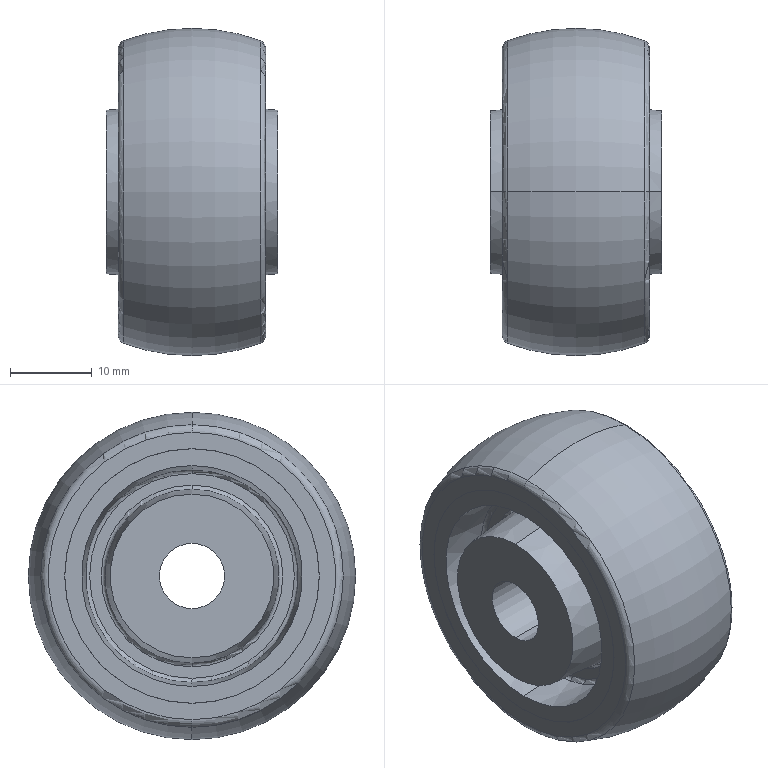Part | STEP file | Frame_top | 1 solid | 42 faces | box 21 x 40 x 40 mm | volume 18711 mm3 | torus 12 | plane 10 | cylinder 10 | cone 8 | other 2 | commonest cylinder face diameters 31.105 x4 31.125 x4 8 x2